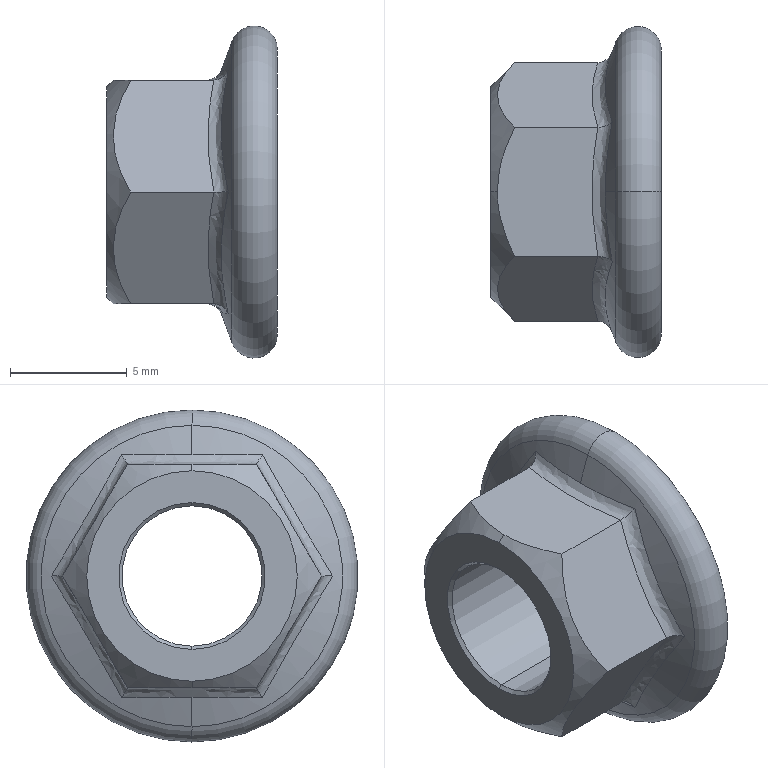Part | SolidWorks | features Cut 2, Boss 1, Chamfer 1, Fillet 1, Revolution 1 | 1 solid | 26 faces | box 7.3 x 14.2 x 14.2 mm | volume 518.031 mm3 | cone 8 | plane 8 | spline 6 | cylinder 2 | torus 2 | commonest cylinder face diameters 6 x2
STEP:
#1=CARTESIAN_POINT('',(-7.3,0.,-4.5));
#2=VERTEX_POINT('',#1);
#3=CARTESIAN_POINT('',(-7.3,0.,4.5));
#4=VERTEX_POINT('',#3);
#5=CARTESIAN_POINT('',(-7.3,0.,0.));
#6=DIRECTION('',(-1.,0.,0.));
#7=DIRECTION('',(0.,0.,1.));
#8=AXIS2_PLACEMENT_3D('',#5,#6,#7);
#9=CIRCLE('',#8,4.5);
#10=EDGE_CURVE('',#2,#4,#9,.T.);
#11=ORIENTED_EDGE('',*,*,#10,.F.);
#12=CARTESIAN_POINT('',(-7.015,0.,-4.785));
#13=VERTEX_POINT('',#12);
#14=CARTESIAN_POINT('',(-7.3,0.,-4.5));
#15=DIRECTION('',(0.7071,0.,-0.7071));
#16=VECTOR('',#15,1000.);
#17=LINE('',#14,#16);
#18=EDGE_CURVE('',#2,#13,#17,.T.);
#19=ORIENTED_EDGE('',*,*,#18,.T.);
#20=CARTESIAN_POINT('',(-6.275,-2.762,-4.785));
#21=VERTEX_POINT('',#20);
#22=CARTESIAN_POINT('',(-7.015,0.,-4.785));
#23=CARTESIAN_POINT('',(-7.015,-0.2426,-4.785));
#24=CARTESIAN_POINT('',(-6.996,-0.4848,-4.785));
#25=CARTESIAN_POINT('',(-6.926,-0.9587,-4.785));
#26=CARTESIAN_POINT('',(-6.874,-1.192,-4.785));
#27=CARTESIAN_POINT('',(-6.677,-1.883,-4.785));
#28=CARTESIAN_POINT('',(-6.489,-2.334,-4.785));
#29=CARTESIAN_POINT('',(-6.275,-2.762,-4.785));
#30=B_SPLINE_CURVE_WITH_KNOTS('',3,(#22,#23,#24,#25,#26,#27,#28,#29),.UNSPECIFIED.,.F.,.F.,(4,2,2,4),(0.005791,0.006506,0.007221,0.008651),.UNSPECIFIED.);
#31=EDGE_CURVE('',#13,#21,#30,.T.);
#32=ORIENTED_EDGE('',*,*,#31,.T.);
#33=CARTESIAN_POINT('',(-6.275,-5.525,0.));
#34=VERTEX_POINT('',#33);
#35=CARTESIAN_POINT('',(-6.275,-2.762,-4.785));
#36=CARTESIAN_POINT('',(-6.491,-2.978,-4.411));
#37=CARTESIAN_POINT('',(-6.674,-3.199,-4.029));
#38=CARTESIAN_POINT('',(-6.871,-3.542,-3.435));
#39=CARTESIAN_POINT('',(-6.923,-3.658,-3.233));
#40=CARTESIAN_POINT('',(-6.995,-3.896,-2.822));
#41=CARTESIAN_POINT('',(-7.015,-4.018,-2.61));
#42=CARTESIAN_POINT('',(-7.016,-4.38,-1.984));
#43=CARTESIAN_POINT('',(-6.943,-4.617,-1.573));
#44=CARTESIAN_POINT('',(-6.678,-5.084,-0.7632));
#45=CARTESIAN_POINT('',(-6.492,-5.308,-0.376));
#46=CARTESIAN_POINT('',(-6.275,-5.525,0.));
#47=B_SPLINE_CURVE_WITH_KNOTS('',3,(#35,#36,#37,#38,#39,#40,#41,#42,#43,#44,#45,#46),.UNSPECIFIED.,.F.,.F.,(4,2,2,2,2,4),(0.000000254,0.001427,0.00214,0.002854,0.004281,0.005707),.UNSPECIFIED.);
#48=EDGE_CURVE('',#21,#34,#47,.T.);
#49=ORIENTED_EDGE('',*,*,#48,.T.);
#50=CARTESIAN_POINT('',(-6.275,-2.763,4.785));
#51=VERTEX_POINT('',#50);
#52=CARTESIAN_POINT('',(-6.275,-5.525,0.));
#53=CARTESIAN_POINT('',(-6.491,-5.309,0.3738));
#54=CARTESIAN_POINT('',(-6.674,-5.088,0.7561));
#55=CARTESIAN_POINT('',(-6.871,-4.746,1.35));
#56=CARTESIAN_POINT('',(-6.923,-4.629,1.551));
#57=CARTESIAN_POINT('',(-6.995,-4.392,1.963));
#58=CARTESIAN_POINT('',(-7.015,-4.269,2.175));
#59=CARTESIAN_POINT('',(-7.016,-3.908,2.801));
#60=CARTESIAN_POINT('',(-6.943,-3.671,3.212));
#61=CARTESIAN_POINT('',(-6.678,-3.203,4.022));
#62=CARTESIAN_POINT('',(-6.492,-2.98,4.409));
#63=CARTESIAN_POINT('',(-6.275,-2.763,4.785));
#64=B_SPLINE_CURVE_WITH_KNOTS('',3,(#52,#53,#54,#55,#56,#57,#58,#59,#60,#61,#62,#63),.UNSPECIFIED.,.F.,.F.,(4,2,2,2,2,4),(0.000000254,0.001427,0.00214,0.002854,0.004281,0.005707),.UNSPECIFIED.);
#65=EDGE_CURVE('',#34,#51,#64,.T.);
#66=ORIENTED_EDGE('',*,*,#65,.T.);
#67=CARTESIAN_POINT('',(-7.015,0.,4.785));
#68=VERTEX_POINT('',#67);
#69=CARTESIAN_POINT('',(-6.275,-2.763,4.785));
#70=CARTESIAN_POINT('',(-6.489,-2.334,4.785));
#71=CARTESIAN_POINT('',(-6.677,-1.883,4.785));
#72=CARTESIAN_POINT('',(-6.874,-1.192,4.785));
#73=CARTESIAN_POINT('',(-6.926,-0.9587,4.785));
#74=CARTESIAN_POINT('',(-6.996,-0.4848,4.785));
#75=CARTESIAN_POINT('',(-7.015,-0.2426,4.785));
#76=CARTESIAN_POINT('',(-7.015,0.,4.785));
#77=B_SPLINE_CURVE_WITH_KNOTS('',3,(#69,#70,#71,#72,#73,#74,#75,#76),.UNSPECIFIED.,.F.,.F.,(4,2,2,4),(0.00366,0.005092,0.005807,0.006523),.UNSPECIFIED.);
#78=EDGE_CURVE('',#51,#68,#77,.T.);
#79=ORIENTED_EDGE('',*,*,#78,.T.);
#80=CARTESIAN_POINT('',(-7.3,0.,4.5));
#81=DIRECTION('',(0.7071,0.,0.7071));
#82=VECTOR('',#81,1000.);
#83=LINE('',#80,#82);
#84=EDGE_CURVE('',#4,#68,#83,.T.);
#85=ORIENTED_EDGE('',*,*,#84,.F.);
#86=EDGE_LOOP('',(#11,#19,#32,#49,#66,#79,#85));
#87=FACE_OUTER_BOUND('',#86,.T.);
#88=CARTESIAN_POINT('',(-7.3,0.,0.));
#89=DIRECTION('',(1.,0.,0.));
#90=DIRECTION('',(0.,0.,1.));
#91=AXIS2_PLACEMENT_3D('',#88,#89,#90);
#92=CONICAL_SURFACE('',#91,4.5,0.7854);
#93=ADVANCED_FACE('',(#87),#92,.T.);
#94=CARTESIAN_POINT('',(-0.1429,0.,3.));
#95=VERTEX_POINT('',#94);
#96=CARTESIAN_POINT('',(-0.1429,0.,-3.));
#97=VERTEX_POINT('',#96);
#98=CARTESIAN_POINT('',(-0.1429,0.,0.));
#99=DIRECTION('',(1.,0.,0.));
#100=DIRECTION('',(0.,0.,1.));
#101=AXIS2_PLACEMENT_3D('',#98,#99,#100);
#102=CIRCLE('',#101,3.);
#103=EDGE_CURVE('',#95,#97,#102,.T.);
#104=ORIENTED_EDGE('',*,*,#103,.F.);
#105=CARTESIAN_POINT('',(0.,0.,3.143));
#106=VERTEX_POINT('',#105);
#107=CARTESIAN_POINT('',(0.,0.,3.143));
#108=DIRECTION('',(0.7071,0.,0.7071));
#109=VECTOR('',#108,1000.);
#110=LINE('',#107,#109);
#111=EDGE_CURVE('',#95,#106,#110,.T.);
#112=ORIENTED_EDGE('',*,*,#111,.T.);
#113=CARTESIAN_POINT('',(0.,0.,-3.143));
#114=VERTEX_POINT('',#113);
#115=CARTESIAN_POINT('',(0.,0.,0.));
#116=DIRECTION('',(-1.,0.,0.));
#117=DIRECTION('',(0.,0.,1.));
#118=AXIS2_PLACEMENT_3D('',#115,#116,#117);
#119=CIRCLE('',#118,3.143);
#120=EDGE_CURVE('',#114,#106,#119,.T.);
#121=ORIENTED_EDGE('',*,*,#120,.F.);
#122=CARTESIAN_POINT('',(0.,0.,-3.143));
#123=DIRECTION('',(0.7071,0.,-0.7071));
#124=VECTOR('',#123,1000.);
#125=LINE('',#122,#124);
#126=EDGE_CURVE('',#97,#114,#125,.T.);
#127=ORIENTED_EDGE('',*,*,#126,.F.);
#128=EDGE_LOOP('',(#104,#112,#121,#127));
#129=FACE_OUTER_BOUND('',#128,.T.);
#130=CARTESIAN_POINT('',(0.,0.,0.));
#131=DIRECTION('',(1.,0.,0.));
#132=DIRECTION('',(0.,0.,-1.));
#133=AXIS2_PLACEMENT_3D('',#130,#131,#132);
#134=CONICAL_SURFACE('',#133,3.143,0.7854);
#135=ADVANCED_FACE('',(#129),#134,.F.);
#136=CARTESIAN_POINT('',(-7.157,0.,-3.));
#137=VERTEX_POINT('',#136);
#138=CARTESIAN_POINT('',(-7.157,0.,3.));
#139=VERTEX_POINT('',#138);
#140=CARTESIAN_POINT('',(-7.157,0.,0.));
#141=DIRECTION('',(-1.,0.,0.));
#142=DIRECTION('',(0.,0.,-1.));
#143=AXIS2_PLACEMENT_3D('',#140,#141,#142);
#144=CIRCLE('',#143,3.);
#145=EDGE_CURVE('',#137,#139,#144,.T.);
#146=ORIENTED_EDGE('',*,*,#145,.F.);
#147=CARTESIAN_POINT('',(-7.3,0.,-3.143));
#148=VERTEX_POINT('',#147);
#149=CARTESIAN_POINT('',(-7.157,0.,-3.));
#150=DIRECTION('',(-0.7071,0.,-0.7071));
#151=VECTOR('',#150,1000.);
#152=LINE('',#149,#151);
#153=EDGE_CURVE('',#137,#148,#152,.T.);
#154=ORIENTED_EDGE('',*,*,#153,.T.);
#155=CARTESIAN_POINT('',(-7.3,0.,3.143));
#156=VERTEX_POINT('',#155);
#157=CARTESIAN_POINT('',(-7.3,0.,0.));
#158=DIRECTION('',(1.,0.,0.));
#159=DIRECTION('',(0.,0.,-1.));
#160=AXIS2_PLACEMENT_3D('',#157,#158,#159);
#161=CIRCLE('',#160,3.143);
#162=EDGE_CURVE('',#156,#148,#161,.T.);
#163=ORIENTED_EDGE('',*,*,#162,.F.);
#164=CARTESIAN_POINT('',(-7.157,0.,3.));
#165=DIRECTION('',(-0.7071,0.,0.7071));
#166=VECTOR('',#165,1000.);
#167=LINE('',#164,#166);
#168=EDGE_CURVE('',#139,#156,#167,.T.);
#169=ORIENTED_EDGE('',*,*,#168,.F.);
#170=EDGE_LOOP('',(#146,#154,#163,#169));
#171=FACE_OUTER_BOUND('',#170,.T.);
#172=CARTESIAN_POINT('',(-7.157,0.,0.));
#173=DIRECTION('',(-1.,0.,0.));
#174=DIRECTION('',(0.,0.,1.));
#175=AXIS2_PLACEMENT_3D('',#172,#173,#174);
#176=CONICAL_SURFACE('',#175,3.,0.7854);
#177=ADVANCED_FACE('',(#171),#176,.F.);
#178=ORIENTED_EDGE('',*,*,#103,.T.);
#179=CARTESIAN_POINT('',(0.,0.,-3.));
#180=DIRECTION('',(-1.,0.,0.));
#181=VECTOR('',#180,1000.);
#182=LINE('',#179,#181);
#183=EDGE_CURVE('',#97,#137,#182,.T.);
#184=ORIENTED_EDGE('',*,*,#183,.T.);
#185=ORIENTED_EDGE('',*,*,#145,.T.);
#186=CARTESIAN_POINT('',(0.,0.,3.));
#187=DIRECTION('',(-1.,0.,0.));
#188=VECTOR('',#187,1000.);
#189=LINE('',#186,#188);
#190=EDGE_CURVE('',#95,#139,#189,.T.);
#191=ORIENTED_EDGE('',*,*,#190,.F.);
#192=EDGE_LOOP('',(#178,#184,#185,#191));
#193=FACE_OUTER_BOUND('',#192,.T.);
#194=CARTESIAN_POINT('',(0.,0.,0.));
#195=DIRECTION('',(-1.,0.,0.));
#196=DIRECTION('',(0.,0.,1.));
#197=AXIS2_PLACEMENT_3D('',#194,#195,#196);
#198=CYLINDRICAL_SURFACE('',#197,3.);
#199=ADVANCED_FACE('',(#193),#198,.F.);
#200=CARTESIAN_POINT('',(0.,0.,6.1));
#201=VERTEX_POINT('',#200);
#202=CARTESIAN_POINT('',(0.,0.,-6.1));
#203=VERTEX_POINT('',#202);
#204=CARTESIAN_POINT('',(0.,0.,0.));
#205=DIRECTION('',(-1.,0.,0.));
#206=DIRECTION('',(0.,0.,1.));
#207=AXIS2_PLACEMENT_3D('',#204,#205,#206);
#208=CIRCLE('',#207,6.1);
#209=EDGE_CURVE('',#201,#203,#208,.T.);
#210=ORIENTED_EDGE('',*,*,#209,.T.);
#211=CARTESIAN_POINT('',(-1.94,0.,-6.442));
#212=VERTEX_POINT('',#211);
#213=CARTESIAN_POINT('',(-1.,0.,-6.1));
#214=DIRECTION('',(0.,1.,0.));
#215=DIRECTION('',(0.,0.,1.));
#216=AXIS2_PLACEMENT_3D('',#213,#214,#215);
#217=CIRCLE('',#216,1.);
#218=EDGE_CURVE('',#203,#212,#217,.T.);
#219=ORIENTED_EDGE('',*,*,#218,.T.);
#220=CARTESIAN_POINT('',(-1.94,0.,6.442));
#221=VERTEX_POINT('',#220);
#222=CARTESIAN_POINT('',(-1.94,0.,0.));
#223=DIRECTION('',(-1.,0.,0.));
#224=DIRECTION('',(0.,0.,1.));
#225=AXIS2_PLACEMENT_3D('',#222,#223,#224);
#226=CIRCLE('',#225,6.442);
#227=EDGE_CURVE('',#221,#212,#226,.T.);
#228=ORIENTED_EDGE('',*,*,#227,.F.);
#229=CARTESIAN_POINT('',(-1.,0.,6.1));
#230=DIRECTION('',(0.,-1.,0.));
#231=DIRECTION('',(0.,0.,-1.));
#232=AXIS2_PLACEMENT_3D('',#229,#230,#231);
#233=CIRCLE('',#232,1.);
#234=EDGE_CURVE('',#201,#221,#233,.T.);
#235=ORIENTED_EDGE('',*,*,#234,.F.);
#236=EDGE_LOOP('',(#210,#219,#228,#235));
#237=FACE_OUTER_BOUND('',#236,.T.);
#238=CARTESIAN_POINT('',(-1.,0.,0.));
#239=DIRECTION('',(-1.,0.,0.));
#240=DIRECTION('',(0.,0.,1.));
#241=AXIS2_PLACEMENT_3D('',#238,#239,#240);
#242=TOROIDAL_SURFACE('',#241,6.1,1.);
#243=ADVANCED_FACE('',(#237),#242,.T.);
#244=CARTESIAN_POINT('',(-2.096,3.006,5.207));
#245=VERTEX_POINT('',#244);
#246=CARTESIAN_POINT('',(-2.399,0.,5.18));
#247=VERTEX_POINT('',#246);
#248=CARTESIAN_POINT('',(-2.096,3.006,5.207));
#249=CARTESIAN_POINT('',(-2.281,2.013,5.193));
#250=CARTESIAN_POINT('',(-2.399,1.012,5.18));
#251=CARTESIAN_POINT('',(-2.399,0.,5.18));
#252=B_SPLINE_CURVE_WITH_KNOTS('',3,(#248,#249,#250,#251),.UNSPECIFIED.,.F.,.F.,(4,4),(0.,0.003022),.UNSPECIFIED.);
#253=EDGE_CURVE('',#245,#247,#252,.T.);
#254=ORIENTED_EDGE('',*,*,#253,.T.);
#255=CARTESIAN_POINT('',(-1.94,0.,6.442));
#256=DIRECTION('',(0.342,0.,0.9397));
#257=VECTOR('',#256,1000.);
#258=LINE('',#255,#257);
#259=EDGE_CURVE('',#247,#221,#258,.T.);
#260=ORIENTED_EDGE('',*,*,#259,.T.);
#261=ORIENTED_EDGE('',*,*,#227,.T.);
#262=CARTESIAN_POINT('',(-2.399,0.,-5.18));
#263=VERTEX_POINT('',#262);
#264=CARTESIAN_POINT('',(-1.94,0.,-6.442));
#265=DIRECTION('',(0.342,0.,-0.9397));
#266=VECTOR('',#265,1000.);
#267=LINE('',#264,#266);
#268=EDGE_CURVE('',#263,#212,#267,.T.);
#269=ORIENTED_EDGE('',*,*,#268,.F.);
#270=CARTESIAN_POINT('',(-2.096,3.006,-5.207));
#271=VERTEX_POINT('',#270);
#272=CARTESIAN_POINT('',(-2.399,0.,-5.18));
#273=CARTESIAN_POINT('',(-2.399,0.5051,-5.18));
#274=CARTESIAN_POINT('',(-2.371,1.008,-5.183));
#275=CARTESIAN_POINT('',(-2.265,2.01,-5.193));
#276=CARTESIAN_POINT('',(-2.189,2.51,-5.2));
#277=CARTESIAN_POINT('',(-2.096,3.006,-5.207));
#278=B_SPLINE_CURVE_WITH_KNOTS('',3,(#272,#273,#274,#275,#276,#277),.UNSPECIFIED.,.F.,.F.,(4,2,4),(0.003022,0.004529,0.006037),.UNSPECIFIED.);
#279=EDGE_CURVE('',#263,#271,#278,.T.);
#280=ORIENTED_EDGE('',*,*,#279,.T.);
#281=CARTESIAN_POINT('',(-2.096,6.013,0.));
#282=VERTEX_POINT('',#281);
#283=CARTESIAN_POINT('',(-2.096,3.006,-5.207));
#284=CARTESIAN_POINT('',(-2.281,3.49,-4.34));
#285=CARTESIAN_POINT('',(-2.399,3.978,-3.468));
#286=CARTESIAN_POINT('',(-2.399,4.737,-2.155));
#287=CARTESIAN_POINT('',(-2.371,4.991,-1.72));
#288=CARTESIAN_POINT('',(-2.265,5.502,-0.8562));
#289=CARTESIAN_POINT('',(-2.189,5.758,-0.4266));
#290=CARTESIAN_POINT('',(-2.096,6.013,0.));
#291=B_SPLINE_CURVE_WITH_KNOTS('',3,(#283,#284,#285,#286,#287,#288,#289,#290),.UNSPECIFIED.,.F.,.F.,(4,2,2,4),(0.,0.003019,0.004528,0.006037),.UNSPECIFIED.);
#292=EDGE_CURVE('',#271,#282,#291,.T.);
#293=ORIENTED_EDGE('',*,*,#292,.T.);
#294=CARTESIAN_POINT('',(-2.096,6.013,0.));
#295=CARTESIAN_POINT('',(-2.281,5.504,0.8523));
#296=CARTESIAN_POINT('',(-2.399,4.993,1.711));
#297=CARTESIAN_POINT('',(-2.399,4.234,3.025));
#298=CARTESIAN_POINT('',(-2.371,3.985,3.463));
#299=CARTESIAN_POINT('',(-2.265,3.492,4.337));
#300=CARTESIAN_POINT('',(-2.189,3.248,4.773));
#301=CARTESIAN_POINT('',(-2.096,3.006,5.207));
#302=B_SPLINE_CURVE_WITH_KNOTS('',3,(#294,#295,#296,#297,#298,#299,#300,#301),.UNSPECIFIED.,.F.,.F.,(4,2,2,4),(0.,0.003019,0.004528,0.006037),.UNSPECIFIED.);
#303=EDGE_CURVE('',#282,#245,#302,.T.);
#304=ORIENTED_EDGE('',*,*,#303,.T.);
#305=EDGE_LOOP('',(#254,#260,#261,#269,#280,#293,#304));
#306=FACE_OUTER_BOUND('',#305,.T.);
#307=CARTESIAN_POINT('',(-1.94,0.,0.));
#308=DIRECTION('',(1.,0.,0.));
#309=DIRECTION('',(0.,0.,-1.));
#310=AXIS2_PLACEMENT_3D('',#307,#308,#309);
#311=CONICAL_SURFACE('',#310,6.442,1.222);
#312=ADVANCED_FACE('',(#306),#311,.T.);
#313=CARTESIAN_POINT('',(-6.275,2.763,4.785));
#314=VERTEX_POINT('',#313);
#315=CARTESIAN_POINT('',(-2.72,2.763,4.785));
#316=VERTEX_POINT('',#315);
#317=CARTESIAN_POINT('',(-7.3,2.763,4.785));
#318=DIRECTION('',(1.,0.,0.));
#319=VECTOR('',#318,1000.);
#320=LINE('',#317,#319);
#321=EDGE_CURVE('',#314,#316,#320,.T.);
#322=ORIENTED_EDGE('',*,*,#321,.T.);
#323=CARTESIAN_POINT('',(-2.72,5.525,0.));
#324=VERTEX_POINT('',#323);
#325=CARTESIAN_POINT('',(-2.72,2.763,4.785));
#326=CARTESIAN_POINT('',(-2.872,3.22,3.993));
#327=CARTESIAN_POINT('',(-2.963,3.68,3.196));
#328=CARTESIAN_POINT('',(-2.963,4.608,1.589));
#329=CARTESIAN_POINT('',(-2.872,5.068,0.7921));
#330=CARTESIAN_POINT('',(-2.72,5.525,0.));
#331=B_SPLINE_CURVE_WITH_KNOTS('',3,(#325,#326,#327,#328,#329,#330),.UNSPECIFIED.,.F.,.F.,(4,2,4),(0.,0.002773,0.005546),.UNSPECIFIED.);
#332=EDGE_CURVE('',#316,#324,#331,.T.);
#333=ORIENTED_EDGE('',*,*,#332,.T.);
#334=CARTESIAN_POINT('',(-6.275,5.525,0.));
#335=VERTEX_POINT('',#334);
#336=CARTESIAN_POINT('',(-7.3,5.525,0.));
#337=DIRECTION('',(1.,0.,0.));
#338=VECTOR('',#337,1000.);
#339=LINE('',#336,#338);
#340=EDGE_CURVE('',#335,#324,#339,.T.);
#341=ORIENTED_EDGE('',*,*,#340,.F.);
#342=CARTESIAN_POINT('',(-6.275,2.763,4.785));
#343=CARTESIAN_POINT('',(-6.491,2.978,4.411));
#344=CARTESIAN_POINT('',(-6.674,3.199,4.029));
#345=CARTESIAN_POINT('',(-6.871,3.542,3.435));
#346=CARTESIAN_POINT('',(-6.923,3.658,3.233));
#347=CARTESIAN_POINT('',(-6.995,3.896,2.822));
#348=CARTESIAN_POINT('',(-7.015,4.018,2.61));
#349=CARTESIAN_POINT('',(-7.016,4.38,1.984));
#350=CARTESIAN_POINT('',(-6.943,4.617,1.573));
#351=CARTESIAN_POINT('',(-6.678,5.084,0.7632));
#352=CARTESIAN_POINT('',(-6.492,5.308,0.376));
#353=CARTESIAN_POINT('',(-6.275,5.525,0.));
#354=B_SPLINE_CURVE_WITH_KNOTS('',3,(#342,#343,#344,#345,#346,#347,#348,#349,#350,#351,#352,#353),.UNSPECIFIED.,.F.,.F.,(4,2,2,2,2,4),(0.000000254,0.001427,0.00214,0.002854,0.004281,0.005707),.UNSPECIFIED.);
#355=EDGE_CURVE('',#314,#335,#354,.T.);
#356=ORIENTED_EDGE('',*,*,#355,.F.);
#357=EDGE_LOOP('',(#322,#333,#341,#356));
#358=FACE_OUTER_BOUND('',#357,.T.);
#359=CARTESIAN_POINT('',(-7.3,2.763,4.785));
#360=DIRECTION('',(0.,-0.866,-0.5));
#361=DIRECTION('',(0.,0.5,-0.866));
#362=AXIS2_PLACEMENT_3D('',#359,#360,#361);
#363=PLANE('',#362);
#364=ADVANCED_FACE('',(#358),#363,.F.);
#365=ORIENTED_EDGE('',*,*,#340,.T.);
#366=CARTESIAN_POINT('',(-2.72,2.763,-4.785));
#367=VERTEX_POINT('',#366);
#368=CARTESIAN_POINT('',(-2.72,5.525,0.));
#369=CARTESIAN_POINT('',(-2.872,5.068,-0.7921));
#370=CARTESIAN_POINT('',(-2.963,4.608,-1.589));
#371=CARTESIAN_POINT('',(-2.963,3.68,-3.196));
#372=CARTESIAN_POINT('',(-2.872,3.22,-3.993));
#373=CARTESIAN_POINT('',(-2.72,2.763,-4.785));
#374=B_SPLINE_CURVE_WITH_KNOTS('',3,(#368,#369,#370,#371,#372,#373),.UNSPECIFIED.,.F.,.F.,(4,2,4),(0.,0.002773,0.005546),.UNSPECIFIED.);
#375=EDGE_CURVE('',#324,#367,#374,.T.);
#376=ORIENTED_EDGE('',*,*,#375,.T.);
#377=CARTESIAN_POINT('',(-6.275,2.763,-4.785));
#378=VERTEX_POINT('',#377);
#379=CARTESIAN_POINT('',(-7.3,2.763,-4.785));
#380=DIRECTION('',(1.,0.,0.));
#381=VECTOR('',#380,1000.);
#382=LINE('',#379,#381);
#383=EDGE_CURVE('',#378,#367,#382,.T.);
#384=ORIENTED_EDGE('',*,*,#383,.F.);
#385=CARTESIAN_POINT('',(-6.275,5.525,0.));
#386=CARTESIAN_POINT('',(-6.491,5.309,-0.3738));
#387=CARTESIAN_POINT('',(-6.674,5.088,-0.7561));
#388=CARTESIAN_POINT('',(-6.871,4.746,-1.35));
#389=CARTESIAN_POINT('',(-6.923,4.629,-1.551));
#390=CARTESIAN_POINT('',(-6.995,4.392,-1.963));
#391=CARTESIAN_POINT('',(-7.015,4.269,-2.175));
#392=CARTESIAN_POINT('',(-7.016,3.908,-2.801));
#393=CARTESIAN_POINT('',(-6.943,3.671,-3.212));
#394=CARTESIAN_POINT('',(-6.678,3.203,-4.022));
#395=CARTESIAN_POINT('',(-6.492,2.98,-4.409));
#396=CARTESIAN_POINT('',(-6.275,2.763,-4.785));
#397=B_SPLINE_CURVE_WITH_KNOTS('',3,(#385,#386,#387,#388,#389,#390,#391,#392,#393,#394,#395,#396),.UNSPECIFIED.,.F.,.F.,(4,2,2,2,2,4),(0.000000254,0.001427,0.00214,0.002854,0.004281,0.005707),.UNSPECIFIED.);
#398=EDGE_CURVE('',#335,#378,#397,.T.);
#399=ORIENTED_EDGE('',*,*,#398,.F.);
#400=EDGE_LOOP('',(#365,#376,#384,#399));
#401=FACE_OUTER_BOUND('',#400,.T.);
#402=CARTESIAN_POINT('',(-7.3,5.525,0.));
#403=DIRECTION('',(0.,-0.866,0.5));
#404=DIRECTION('',(0.,-0.5,-0.866));
#405=AXIS2_PLACEMENT_3D('',#402,#403,#404);
#406=PLANE('',#405);
#407=ADVANCED_FACE('',(#401),#406,.F.);
#408=ORIENTED_EDGE('',*,*,#383,.T.);
#409=CARTESIAN_POINT('',(-2.72,-2.762,-4.785));
#410=VERTEX_POINT('',#409);
#411=CARTESIAN_POINT('',(-2.72,2.763,-4.785));
#412=CARTESIAN_POINT('',(-2.872,1.848,-4.785));
#413=CARTESIAN_POINT('',(-2.963,0.9279,-4.785));
#414=CARTESIAN_POINT('',(-2.963,-0.928,-4.785));
#415=CARTESIAN_POINT('',(-2.872,-1.848,-4.785));
#416=CARTESIAN_POINT('',(-2.72,-2.762,-4.785));
#417=B_SPLINE_CURVE_WITH_KNOTS('',3,(#411,#412,#413,#414,#415,#416),.UNSPECIFIED.,.F.,.F.,(4,2,4),(0.,0.002773,0.005546),.UNSPECIFIED.);
#418=EDGE_CURVE('',#367,#410,#417,.T.);
#419=ORIENTED_EDGE('',*,*,#418,.T.);
#420=CARTESIAN_POINT('',(-7.3,-2.762,-4.785));
#421=DIRECTION('',(1.,0.,0.));
#422=VECTOR('',#421,1000.);
#423=LINE('',#420,#422);
#424=EDGE_CURVE('',#21,#410,#423,.T.);
#425=ORIENTED_EDGE('',*,*,#424,.F.);
#426=ORIENTED_EDGE('',*,*,#31,.F.);
#427=CARTESIAN_POINT('',(-6.275,2.763,-4.785));
#428=CARTESIAN_POINT('',(-6.382,2.549,-4.785));
#429=CARTESIAN_POINT('',(-6.482,2.331,-4.785));
#430=CARTESIAN_POINT('',(-6.662,1.884,-4.785));
#431=CARTESIAN_POINT('',(-6.742,1.653,-4.785));
#432=CARTESIAN_POINT('',(-6.94,0.9586,-4.785));
#433=CARTESIAN_POINT('',(-7.015,0.4856,-4.785));
#434=CARTESIAN_POINT('',(-7.015,0.,-4.785));
#435=B_SPLINE_CURVE_WITH_KNOTS('',3,(#427,#428,#429,#430,#431,#432,#433,#434),.UNSPECIFIED.,.F.,.F.,(4,2,2,4),(0.002927,0.003643,0.004359,0.005791),.UNSPECIFIED.);
#436=EDGE_CURVE('',#378,#13,#435,.T.);
#437=ORIENTED_EDGE('',*,*,#436,.F.);
#438=EDGE_LOOP('',(#408,#419,#425,#426,#437));
#439=FACE_OUTER_BOUND('',#438,.T.);
#440=CARTESIAN_POINT('',(-7.3,2.763,-4.785));
#441=DIRECTION('',(0.,0.,1.));
#442=DIRECTION('',(0.,-1.,0.));
#443=AXIS2_PLACEMENT_3D('',#440,#441,#442);
#444=PLANE('',#443);
#445=ADVANCED_FACE('',(#439),#444,.F.);
#446=ORIENTED_EDGE('',*,*,#424,.T.);
#447=CARTESIAN_POINT('',(-2.72,-5.525,0.));
#448=VERTEX_POINT('',#447);
#449=CARTESIAN_POINT('',(-2.72,-2.762,-4.785));
#450=CARTESIAN_POINT('',(-2.872,-3.22,-3.993));
#451=CARTESIAN_POINT('',(-2.963,-3.68,-3.196));
#452=CARTESIAN_POINT('',(-2.963,-4.608,-1.589));
#453=CARTESIAN_POINT('',(-2.872,-5.068,-0.7921));
#454=CARTESIAN_POINT('',(-2.72,-5.525,0.));
#455=B_SPLINE_CURVE_WITH_KNOTS('',3,(#449,#450,#451,#452,#453,#454),.UNSPECIFIED.,.F.,.F.,(4,2,4),(0.,0.002773,0.005546),.UNSPECIFIED.);
#456=EDGE_CURVE('',#410,#448,#455,.T.);
#457=ORIENTED_EDGE('',*,*,#456,.T.);
#458=CARTESIAN_POINT('',(-7.3,-5.525,0.));
#459=DIRECTION('',(1.,0.,0.));
#460=VECTOR('',#459,1000.);
#461=LINE('',#458,#460);
#462=EDGE_CURVE('',#34,#448,#461,.T.);
#463=ORIENTED_EDGE('',*,*,#462,.F.);
#464=ORIENTED_EDGE('',*,*,#48,.F.);
#465=EDGE_LOOP('',(#446,#457,#463,#464));
#466=FACE_OUTER_BOUND('',#465,.T.);
#467=CARTESIAN_POINT('',(-7.3,-2.762,-4.785));
#468=DIRECTION('',(0.,0.866,0.5));
#469=DIRECTION('',(0.,-0.5,0.866));
#470=AXIS2_PLACEMENT_3D('',#467,#468,#469);
#471=PLANE('',#470);
#472=ADVANCED_FACE('',(#466),#471,.F.);
#473=ORIENTED_EDGE('',*,*,#462,.T.);
#474=CARTESIAN_POINT('',(-2.72,-2.763,4.785));
#475=VERTEX_POINT('',#474);
#476=CARTESIAN_POINT('',(-2.72,-5.525,0.));
#477=CARTESIAN_POINT('',(-2.872,-5.068,0.7921));
#478=CARTESIAN_POINT('',(-2.963,-4.608,1.589));
#479=CARTESIAN_POINT('',(-2.963,-3.68,3.196));
#480=CARTESIAN_POINT('',(-2.872,-3.22,3.993));
#481=CARTESIAN_POINT('',(-2.72,-2.763,4.785));
#482=B_SPLINE_CURVE_WITH_KNOTS('',3,(#476,#477,#478,#479,#480,#481),.UNSPECIFIED.,.F.,.F.,(4,2,4),(0.,0.002773,0.005546),.UNSPECIFIED.);
#483=EDGE_CURVE('',#448,#475,#482,.T.);
#484=ORIENTED_EDGE('',*,*,#483,.T.);
#485=CARTESIAN_POINT('',(-7.3,-2.763,4.785));
#486=DIRECTION('',(1.,0.,0.));
#487=VECTOR('',#486,1000.);
#488=LINE('',#485,#487);
#489=EDGE_CURVE('',#51,#475,#488,.T.);
#490=ORIENTED_EDGE('',*,*,#489,.F.);
#491=ORIENTED_EDGE('',*,*,#65,.F.);
#492=EDGE_LOOP('',(#473,#484,#490,#491));
#493=FACE_OUTER_BOUND('',#492,.T.);
#494=CARTESIAN_POINT('',(-7.3,-5.525,0.));
#495=DIRECTION('',(0.,0.866,-0.5));
#496=DIRECTION('',(0.,0.5,0.866));
#497=AXIS2_PLACEMENT_3D('',#494,#495,#496);
#498=PLANE('',#497);
#499=ADVANCED_FACE('',(#493),#498,.F.);
#500=ORIENTED_EDGE('',*,*,#489,.T.);
#501=CARTESIAN_POINT('',(-2.72,-2.763,4.785));
#502=CARTESIAN_POINT('',(-2.872,-1.848,4.785));
#503=CARTESIAN_POINT('',(-2.963,-0.928,4.785));
#504=CARTESIAN_POINT('',(-2.963,0.9279,4.785));
#505=CARTESIAN_POINT('',(-2.872,1.848,4.785));
#506=CARTESIAN_POINT('',(-2.72,2.763,4.785));
#507=B_SPLINE_CURVE_WITH_KNOTS('',3,(#501,#502,#503,#504,#505,#506),.UNSPECIFIED.,.F.,.F.,(4,2,4),(0.,0.002773,0.005546),.UNSPECIFIED.);
#508=EDGE_CURVE('',#475,#316,#507,.T.);
#509=ORIENTED_EDGE('',*,*,#508,.T.);
#510=ORIENTED_EDGE('',*,*,#321,.F.);
#511=CARTESIAN_POINT('',(-7.015,0.,4.785));
#512=CARTESIAN_POINT('',(-7.015,0.4856,4.785));
#513=CARTESIAN_POINT('',(-6.94,0.9586,4.785));
#514=CARTESIAN_POINT('',(-6.742,1.653,4.785));
#515=CARTESIAN_POINT('',(-6.662,1.884,4.785));
#516=CARTESIAN_POINT('',(-6.482,2.331,4.785));
#517=CARTESIAN_POINT('',(-6.382,2.549,4.785));
#518=CARTESIAN_POINT('',(-6.275,2.763,4.785));
#519=B_SPLINE_CURVE_WITH_KNOTS('',3,(#511,#512,#513,#514,#515,#516,#517,#518),.UNSPECIFIED.,.F.,.F.,(4,2,2,4),(0.006523,0.007956,0.008672,0.009389),.UNSPECIFIED.);
#520=EDGE_CURVE('',#68,#314,#519,.T.);
#521=ORIENTED_EDGE('',*,*,#520,.F.);
#522=ORIENTED_EDGE('',*,*,#78,.F.);
#523=EDGE_LOOP('',(#500,#509,#510,#521,#522));
#524=FACE_OUTER_BOUND('',#523,.T.);
#525=CARTESIAN_POINT('',(-7.3,-2.763,4.785));
#526=DIRECTION('',(0.,0.,-1.));
#527=DIRECTION('',(0.,1.,0.));
#528=AXIS2_PLACEMENT_3D('',#525,#526,#527);
#529=PLANE('',#528);
#530=ADVANCED_FACE('',(#524),#529,.F.);
#531=ORIENTED_EDGE('',*,*,#162,.T.);
#532=CARTESIAN_POINT('',(-7.3,0.,0.));
#533=DIRECTION('',(1.,0.,0.));
#534=DIRECTION('',(0.,0.,-1.));
#535=AXIS2_PLACEMENT_3D('',#532,#533,#534);
#536=CIRCLE('',#535,3.143);
#537=EDGE_CURVE('',#148,#156,#536,.T.);
#538=ORIENTED_EDGE('',*,*,#537,.T.);
#539=EDGE_LOOP('',(#531,#538));
#540=FACE_BOUND('',#539,.T.);
#541=CARTESIAN_POINT('',(-7.3,0.,0.));
#542=DIRECTION('',(-1.,0.,0.));
#543=DIRECTION('',(0.,0.,1.));
#544=AXIS2_PLACEMENT_3D('',#541,#542,#543);
#545=CIRCLE('',#544,4.5);
#546=EDGE_CURVE('',#4,#2,#545,.T.);
#547=ORIENTED_EDGE('',*,*,#546,.T.);
#548=ORIENTED_EDGE('',*,*,#10,.T.);
#549=EDGE_LOOP('',(#547,#548));
#550=FACE_OUTER_BOUND('',#549,.T.);
#551=CARTESIAN_POINT('',(-7.3,2.763,4.785));
#552=DIRECTION('',(1.,0.,0.));
#553=DIRECTION('',(0.,0.,-1.));
#554=AXIS2_PLACEMENT_3D('',#551,#552,#553);
#555=PLANE('',#554);
#556=ADVANCED_FACE('',(#540,#550),#555,.F.);
#557=ORIENTED_EDGE('',*,*,#259,.F.);
#558=CARTESIAN_POINT('',(-2.096,-3.006,5.207));
#559=VERTEX_POINT('',#558);
#560=CARTESIAN_POINT('',(-2.399,0.,5.18));
#561=CARTESIAN_POINT('',(-2.399,-0.5052,5.18));
#562=CARTESIAN_POINT('',(-2.371,-1.008,5.183));
#563=CARTESIAN_POINT('',(-2.265,-2.01,5.193));
#564=CARTESIAN_POINT('',(-2.189,-2.51,5.2));
#565=CARTESIAN_POINT('',(-2.096,-3.006,5.207));
#566=B_SPLINE_CURVE_WITH_KNOTS('',3,(#560,#561,#562,#563,#564,#565),.UNSPECIFIED.,.F.,.F.,(4,2,4),(0.003022,0.004529,0.006037),.UNSPECIFIED.);
#567=EDGE_CURVE('',#247,#559,#566,.T.);
#568=ORIENTED_EDGE('',*,*,#567,.T.);
#569=CARTESIAN_POINT('',(-2.096,-6.013,0.));
#570=VERTEX_POINT('',#569);
#571=CARTESIAN_POINT('',(-2.096,-3.006,5.207));
#572=CARTESIAN_POINT('',(-2.281,-3.49,4.34));
#573=CARTESIAN_POINT('',(-2.399,-3.978,3.468));
#574=CARTESIAN_POINT('',(-2.399,-4.737,2.155));
#575=CARTESIAN_POINT('',(-2.371,-4.991,1.72));
#576=CARTESIAN_POINT('',(-2.265,-5.502,0.8562));
#577=CARTESIAN_POINT('',(-2.189,-5.758,0.4266));
#578=CARTESIAN_POINT('',(-2.096,-6.013,0.));
#579=B_SPLINE_CURVE_WITH_KNOTS('',3,(#571,#572,#573,#574,#575,#576,#577,#578),.UNSPECIFIED.,.F.,.F.,(4,2,2,4),(0.,0.003019,0.004528,0.006037),.UNSPECIFIED.);
#580=EDGE_CURVE('',#559,#570,#579,.T.);
#581=ORIENTED_EDGE('',*,*,#580,.T.);
#582=CARTESIAN_POINT('',(-2.096,-3.006,-5.207));
#583=VERTEX_POINT('',#582);
#584=CARTESIAN_POINT('',(-2.096,-6.013,0.));
#585=CARTESIAN_POINT('',(-2.281,-5.504,-0.8523));
#586=CARTESIAN_POINT('',(-2.399,-4.993,-1.711));
#587=CARTESIAN_POINT('',(-2.399,-4.234,-3.025));
#588=CARTESIAN_POINT('',(-2.371,-3.985,-3.463));
#589=CARTESIAN_POINT('',(-2.265,-3.492,-4.337));
#590=CARTESIAN_POINT('',(-2.189,-3.248,-4.773));
#591=CARTESIAN_POINT('',(-2.096,-3.006,-5.207));
#592=B_SPLINE_CURVE_WITH_KNOTS('',3,(#584,#585,#586,#587,#588,#589,#590,#591),.UNSPECIFIED.,.F.,.F.,(4,2,2,4),(0.,0.003019,0.004528,0.006037),.UNSPECIFIED.);
#593=EDGE_CURVE('',#570,#583,#592,.T.);
#594=ORIENTED_EDGE('',*,*,#593,.T.);
#595=CARTESIAN_POINT('',(-2.096,-3.006,-5.207));
#596=CARTESIAN_POINT('',(-2.281,-2.013,-5.193));
#597=CARTESIAN_POINT('',(-2.399,-1.012,-5.18));
#598=CARTESIAN_POINT('',(-2.399,0.,-5.18));
#599=B_SPLINE_CURVE_WITH_KNOTS('',3,(#595,#596,#597,#598),.UNSPECIFIED.,.F.,.F.,(4,4),(0.,0.003022),.UNSPECIFIED.);
#600=EDGE_CURVE('',#583,#263,#599,.T.);
#601=ORIENTED_EDGE('',*,*,#600,.T.);
#602=ORIENTED_EDGE('',*,*,#268,.T.);
#603=CARTESIAN_POINT('',(-1.94,0.,0.));
#604=DIRECTION('',(-1.,0.,0.));
#605=DIRECTION('',(0.,0.,1.));
#606=AXIS2_PLACEMENT_3D('',#603,#604,#605);
#607=CIRCLE('',#606,6.442);
#608=EDGE_CURVE('',#212,#221,#607,.T.);
#609=ORIENTED_EDGE('',*,*,#608,.T.);
#610=EDGE_LOOP('',(#557,#568,#581,#594,#601,#602,#609));
#611=FACE_OUTER_BOUND('',#610,.T.);
#612=CARTESIAN_POINT('',(-1.94,0.,0.));
#613=DIRECTION('',(1.,0.,0.));
#614=DIRECTION('',(0.,0.,-1.));
#615=AXIS2_PLACEMENT_3D('',#612,#613,#614);
#616=CONICAL_SURFACE('',#615,6.442,1.222);
#617=ADVANCED_FACE('',(#611),#616,.T.);
#618=ORIENTED_EDGE('',*,*,#120,.T.);
#619=CARTESIAN_POINT('',(0.,0.,0.));
#620=DIRECTION('',(-1.,0.,0.));
#621=DIRECTION('',(0.,0.,1.));
#622=AXIS2_PLACEMENT_3D('',#619,#620,#621);
#623=CIRCLE('',#622,3.143);
#624=EDGE_CURVE('',#106,#114,#623,.T.);
#625=ORIENTED_EDGE('',*,*,#624,.T.);
#626=EDGE_LOOP('',(#618,#625));
#627=FACE_BOUND('',#626,.T.);
#628=ORIENTED_EDGE('',*,*,#209,.F.);
#629=CARTESIAN_POINT('',(0.,0.,0.));
#630=DIRECTION('',(-1.,0.,0.));
#631=DIRECTION('',(0.,0.,1.));
#632=AXIS2_PLACEMENT_3D('',#629,#630,#631);
#633=CIRCLE('',#632,6.1);
#634=EDGE_CURVE('',#203,#201,#633,.T.);
#635=ORIENTED_EDGE('',*,*,#634,.F.);
#636=EDGE_LOOP('',(#628,#635));
#637=FACE_OUTER_BOUND('',#636,.T.);
#638=CARTESIAN_POINT('',(0.,0.,0.));
#639=DIRECTION('',(-1.,0.,0.));
#640=DIRECTION('',(0.,0.,1.));
#641=AXIS2_PLACEMENT_3D('',#638,#639,#640);
#642=PLANE('',#641);
#643=ADVANCED_FACE('',(#627,#637),#642,.F.);
#644=ORIENTED_EDGE('',*,*,#218,.F.);
#645=ORIENTED_EDGE('',*,*,#634,.T.);
#646=ORIENTED_EDGE('',*,*,#234,.T.);
#647=ORIENTED_EDGE('',*,*,#608,.F.);
#648=EDGE_LOOP('',(#644,#645,#646,#647));
#649=FACE_OUTER_BOUND('',#648,.T.);
#650=CARTESIAN_POINT('',(-1.,0.,0.));
#651=DIRECTION('',(-1.,0.,0.));
#652=DIRECTION('',(0.,0.,1.));
#653=AXIS2_PLACEMENT_3D('',#650,#651,#652);
#654=TOROIDAL_SURFACE('',#653,6.1,1.);
#655=ADVANCED_FACE('',(#649),#654,.T.);
#656=ORIENTED_EDGE('',*,*,#183,.F.);
#657=CARTESIAN_POINT('',(-0.1429,0.,0.));
#658=DIRECTION('',(1.,0.,0.));
#659=DIRECTION('',(0.,0.,1.));
#660=AXIS2_PLACEMENT_3D('',#657,#658,#659);
#661=CIRCLE('',#660,3.);
#662=EDGE_CURVE('',#97,#95,#661,.T.);
#663=ORIENTED_EDGE('',*,*,#662,.T.);
#664=ORIENTED_EDGE('',*,*,#190,.T.);
#665=CARTESIAN_POINT('',(-7.157,0.,0.));
#666=DIRECTION('',(-1.,0.,0.));
#667=DIRECTION('',(0.,0.,-1.));
#668=AXIS2_PLACEMENT_3D('',#665,#666,#667);
#669=CIRCLE('',#668,3.);
#670=EDGE_CURVE('',#139,#137,#669,.T.);
#671=ORIENTED_EDGE('',*,*,#670,.T.);
#672=EDGE_LOOP('',(#656,#663,#664,#671));
#673=FACE_OUTER_BOUND('',#672,.T.);
#674=CARTESIAN_POINT('',(0.,0.,0.));
#675=DIRECTION('',(-1.,0.,0.));
#676=DIRECTION('',(0.,0.,1.));
#677=AXIS2_PLACEMENT_3D('',#674,#675,#676);
#678=CYLINDRICAL_SURFACE('',#677,3.);
#679=ADVANCED_FACE('',(#673),#678,.F.);
#680=ORIENTED_EDGE('',*,*,#153,.F.);
#681=ORIENTED_EDGE('',*,*,#670,.F.);
#682=ORIENTED_EDGE('',*,*,#168,.T.);
#683=ORIENTED_EDGE('',*,*,#537,.F.);
#684=EDGE_LOOP('',(#680,#681,#682,#683));
#685=FACE_OUTER_BOUND('',#684,.T.);
#686=CARTESIAN_POINT('',(-7.157,0.,0.));
#687=DIRECTION('',(-1.,0.,0.));
#688=DIRECTION('',(0.,0.,1.));
#689=AXIS2_PLACEMENT_3D('',#686,#687,#688);
#690=CONICAL_SURFACE('',#689,3.,0.7854);
#691=ADVANCED_FACE('',(#685),#690,.F.);
#692=ORIENTED_EDGE('',*,*,#111,.F.);
#693=ORIENTED_EDGE('',*,*,#662,.F.);
#694=ORIENTED_EDGE('',*,*,#126,.T.);
#695=ORIENTED_EDGE('',*,*,#624,.F.);
#696=EDGE_LOOP('',(#692,#693,#694,#695));
#697=FACE_OUTER_BOUND('',#696,.T.);
#698=CARTESIAN_POINT('',(0.,0.,0.));
#699=DIRECTION('',(1.,0.,0.));
#700=DIRECTION('',(0.,0.,-1.));
#701=AXIS2_PLACEMENT_3D('',#698,#699,#700);
#702=CONICAL_SURFACE('',#701,3.143,0.7854);
#703=ADVANCED_FACE('',(#697),#702,.F.);
#704=ORIENTED_EDGE('',*,*,#18,.F.);
#705=ORIENTED_EDGE('',*,*,#546,.F.);
#706=ORIENTED_EDGE('',*,*,#84,.T.);
#707=ORIENTED_EDGE('',*,*,#520,.T.);
#708=ORIENTED_EDGE('',*,*,#355,.T.);
#709=ORIENTED_EDGE('',*,*,#398,.T.);
#710=ORIENTED_EDGE('',*,*,#436,.T.);
#711=EDGE_LOOP('',(#704,#705,#706,#707,#708,#709,#710));
#712=FACE_OUTER_BOUND('',#711,.T.);
#713=CARTESIAN_POINT('',(-7.3,0.,0.));
#714=DIRECTION('',(1.,0.,0.));
#715=DIRECTION('',(0.,0.,1.));
#716=AXIS2_PLACEMENT_3D('',#713,#714,#715);
#717=CONICAL_SURFACE('',#716,4.5,0.7854);
#718=ADVANCED_FACE('',(#712),#717,.T.);
#719=CARTESIAN_POINT('',(-2.096,-6.013,0.));
#720=CARTESIAN_POINT('',(-2.144,-5.881,0.));
#721=CARTESIAN_POINT('',(-2.225,-5.761,0.));
#722=CARTESIAN_POINT('',(-2.443,-5.582,0.));
#723=CARTESIAN_POINT('',(-2.578,-5.525,0.));
#724=CARTESIAN_POINT('',(-2.72,-5.525,0.));
#725=B_SPLINE_CURVE_WITH_KNOTS('',3,(#719,#720,#721,#722,#723,#724),.UNSPECIFIED.,.F.,.F.,(4,2,4),(-0.000005124,0.000415,0.000835),.UNSPECIFIED.);
#726=EDGE_CURVE('',#570,#448,#725,.T.);
#727=ORIENTED_EDGE('',*,*,#726,.F.);
#728=ORIENTED_EDGE('',*,*,#580,.F.);
#729=CARTESIAN_POINT('',(-2.72,-2.763,4.785));
#730=CARTESIAN_POINT('',(-2.578,-2.763,4.785));
#731=CARTESIAN_POINT('',(-2.443,-2.791,4.834));
#732=CARTESIAN_POINT('',(-2.225,-2.88,4.989));
#733=CARTESIAN_POINT('',(-2.144,-2.941,5.094));
#734=CARTESIAN_POINT('',(-2.096,-3.006,5.207));
#735=B_SPLINE_CURVE_WITH_KNOTS('',3,(#729,#730,#731,#732,#733,#734),.UNSPECIFIED.,.F.,.F.,(4,2,4),(0.,0.0004186,0.0008372),.UNSPECIFIED.);
#736=EDGE_CURVE('',#475,#559,#735,.T.);
#737=ORIENTED_EDGE('',*,*,#736,.F.);
#738=ORIENTED_EDGE('',*,*,#483,.F.);
#739=EDGE_LOOP('',(#727,#728,#737,#738));
#740=FACE_OUTER_BOUND('',#739,.T.);
#741=CARTESIAN_POINT('',(-2.089,-2.989,5.238));
#742=CARTESIAN_POINT('',(-2.218,-2.611,5.047));
#743=CARTESIAN_POINT('',(-2.653,-2.571,5.116));
#744=CARTESIAN_POINT('',(-2.276,-3.472,4.372));
#745=CARTESIAN_POINT('',(-2.411,-3.104,4.193));
#746=CARTESIAN_POINT('',(-2.84,-3.079,4.236));
#747=CARTESIAN_POINT('',(-2.398,-3.96,3.501));
#748=CARTESIAN_POINT('',(-2.541,-3.612,3.313));
#749=CARTESIAN_POINT('',(-2.961,-3.597,3.339));
#750=CARTESIAN_POINT('',(-2.401,-4.99,1.716));
#751=CARTESIAN_POINT('',(-2.545,-4.653,1.509));
#752=CARTESIAN_POINT('',(-2.965,-4.668,1.484));
#753=CARTESIAN_POINT('',(-2.281,-5.51,0.8425));
#754=CARTESIAN_POINT('',(-2.416,-5.171,0.613));
#755=CARTESIAN_POINT('',(-2.844,-5.196,0.5703));
#756=CARTESIAN_POINT('',(-2.089,-6.031,-0.03106));
#757=CARTESIAN_POINT('',(-2.218,-5.677,-0.2629));
#758=CARTESIAN_POINT('',(-2.653,-5.717,-0.3321));
#759=(BOUNDED_SURFACE()B_SPLINE_SURFACE(3,2,((#741,#742,#743),(#744,#745,#746),(#747,#748,#749),(#750,#751,#752),(#753,#754,#755),(#756,#757,#758)),.UNSPECIFIED.,.F.,.F.,.F.)B_SPLINE_SURFACE_WITH_KNOTS((4,2,4),(3,3),(0.0256,0.02868,0.03176),(0.,1.),.UNSPECIFIED.)GEOMETRIC_REPRESENTATION_ITEM()RATIONAL_B_SPLINE_SURFACE(((1.,0.8048,1.),(1.,0.8124,1.),(1.,0.8191,1.),(1.,0.8192,1.),(1.,0.8126,1.),(1.,0.8048,1.)))REPRESENTATION_ITEM('')SURFACE());
#760=ADVANCED_FACE('',(#740),#759,.F.);
#761=ORIENTED_EDGE('',*,*,#736,.T.);
#762=ORIENTED_EDGE('',*,*,#567,.F.);
#763=ORIENTED_EDGE('',*,*,#253,.F.);
#764=CARTESIAN_POINT('',(-2.72,2.763,4.785));
#765=CARTESIAN_POINT('',(-2.578,2.762,4.785));
#766=CARTESIAN_POINT('',(-2.443,2.791,4.834));
#767=CARTESIAN_POINT('',(-2.225,2.88,4.989));
#768=CARTESIAN_POINT('',(-2.144,2.941,5.094));
#769=CARTESIAN_POINT('',(-2.096,3.006,5.207));
#770=B_SPLINE_CURVE_WITH_KNOTS('',3,(#764,#765,#766,#767,#768,#769),.UNSPECIFIED.,.F.,.F.,(4,2,4),(0.,0.0004186,0.0008372),.UNSPECIFIED.);
#771=EDGE_CURVE('',#316,#245,#770,.T.);
#772=ORIENTED_EDGE('',*,*,#771,.F.);
#773=ORIENTED_EDGE('',*,*,#508,.F.);
#774=EDGE_LOOP('',(#761,#762,#763,#772,#773));
#775=FACE_OUTER_BOUND('',#774,.T.);
#776=CARTESIAN_POINT('',(-2.089,3.042,5.208));
#777=CARTESIAN_POINT('',(-2.218,3.065,4.785));
#778=CARTESIAN_POINT('',(-2.653,3.145,4.785));
#779=CARTESIAN_POINT('',(-2.276,2.05,5.193));
#780=CARTESIAN_POINT('',(-2.411,2.079,4.785));
#781=CARTESIAN_POINT('',(-2.84,2.129,4.785));
#782=CARTESIAN_POINT('',(-2.398,1.052,5.18));
#783=CARTESIAN_POINT('',(-2.541,1.062,4.785));
#784=CARTESIAN_POINT('',(-2.961,1.093,4.785));
#785=CARTESIAN_POINT('',(-2.401,-1.01,5.179));
#786=CARTESIAN_POINT('',(-2.545,-1.02,4.785));
#787=CARTESIAN_POINT('',(-2.965,-1.05,4.785));
#788=CARTESIAN_POINT('',(-2.281,-2.025,5.193));
#789=CARTESIAN_POINT('',(-2.416,-2.055,4.785));
#790=CARTESIAN_POINT('',(-2.844,-2.104,4.785));
#791=CARTESIAN_POINT('',(-2.089,-3.042,5.208));
#792=CARTESIAN_POINT('',(-2.218,-3.066,4.785));
#793=CARTESIAN_POINT('',(-2.653,-3.146,4.785));
#794=(BOUNDED_SURFACE()B_SPLINE_SURFACE(3,2,((#776,#777,#778),(#779,#780,#781),(#782,#783,#784),(#785,#786,#787),(#788,#789,#790),(#791,#792,#793)),.UNSPECIFIED.,.F.,.F.,.F.)B_SPLINE_SURFACE_WITH_KNOTS((4,2,4),(3,3),(0.02553,0.02861,0.03169),(0.,1.),.UNSPECIFIED.)GEOMETRIC_REPRESENTATION_ITEM()RATIONAL_B_SPLINE_SURFACE(((1.,0.8048,1.),(1.,0.8124,1.),(1.,0.8191,1.),(1.,0.8192,1.),(1.,0.8126,1.),(1.,0.8048,1.)))REPRESENTATION_ITEM('')SURFACE());
#795=ADVANCED_FACE('',(#775),#794,.F.);
#796=ORIENTED_EDGE('',*,*,#726,.T.);
#797=ORIENTED_EDGE('',*,*,#456,.F.);
#798=CARTESIAN_POINT('',(-2.096,-3.006,-5.207));
#799=CARTESIAN_POINT('',(-2.144,-2.941,-5.093));
#800=CARTESIAN_POINT('',(-2.225,-2.88,-4.989));
#801=CARTESIAN_POINT('',(-2.443,-2.791,-4.834));
#802=CARTESIAN_POINT('',(-2.578,-2.762,-4.785));
#803=CARTESIAN_POINT('',(-2.72,-2.762,-4.785));
#804=B_SPLINE_CURVE_WITH_KNOTS('',3,(#798,#799,#800,#801,#802,#803),.UNSPECIFIED.,.F.,.F.,(4,2,4),(-0.000005124,0.000415,0.000835),.UNSPECIFIED.);
#805=EDGE_CURVE('',#583,#410,#804,.T.);
#806=ORIENTED_EDGE('',*,*,#805,.F.);
#807=ORIENTED_EDGE('',*,*,#593,.F.);
#808=EDGE_LOOP('',(#796,#797,#806,#807));
#809=FACE_OUTER_BOUND('',#808,.T.);
#810=CARTESIAN_POINT('',(-2.089,-6.031,0.03028));
#811=CARTESIAN_POINT('',(-2.218,-5.676,0.2621));
#812=CARTESIAN_POINT('',(-2.653,-5.716,0.3313));
#813=CARTESIAN_POINT('',(-2.276,-5.522,-0.8215));
#814=CARTESIAN_POINT('',(-2.411,-5.183,-0.5921));
#815=CARTESIAN_POINT('',(-2.84,-5.208,-0.5485));
#816=CARTESIAN_POINT('',(-2.398,-5.012,-1.679));
#817=CARTESIAN_POINT('',(-2.541,-4.675,-1.472));
#818=CARTESIAN_POINT('',(-2.961,-4.691,-1.445));
#819=CARTESIAN_POINT('',(-2.401,-3.981,-3.464));
#820=CARTESIAN_POINT('',(-2.545,-3.634,-3.275));
#821=CARTESIAN_POINT('',(-2.965,-3.619,-3.301));
#822=CARTESIAN_POINT('',(-2.281,-3.484,-4.35));
#823=CARTESIAN_POINT('',(-2.416,-3.116,-4.172));
#824=CARTESIAN_POINT('',(-2.844,-3.092,-4.215));
#825=CARTESIAN_POINT('',(-2.089,-2.989,-5.239));
#826=CARTESIAN_POINT('',(-2.218,-2.611,-5.048));
#827=CARTESIAN_POINT('',(-2.653,-2.571,-5.117));
#828=(BOUNDED_SURFACE()B_SPLINE_SURFACE(3,2,((#810,#811,#812),(#813,#814,#815),(#816,#817,#818),(#819,#820,#821),(#822,#823,#824),(#825,#826,#827)),.UNSPECIFIED.,.F.,.F.,.F.)B_SPLINE_SURFACE_WITH_KNOTS((4,2,4),(3,3),(0.0256,0.02868,0.03176),(0.,1.),.UNSPECIFIED.)GEOMETRIC_REPRESENTATION_ITEM()RATIONAL_B_SPLINE_SURFACE(((1.,0.8048,1.),(1.,0.8124,1.),(1.,0.8191,1.),(1.,0.8192,1.),(1.,0.8126,1.),(1.,0.8048,1.)))REPRESENTATION_ITEM('')SURFACE());
#829=ADVANCED_FACE('',(#809),#828,.F.);
#830=ORIENTED_EDGE('',*,*,#771,.T.);
#831=ORIENTED_EDGE('',*,*,#303,.F.);
#832=CARTESIAN_POINT('',(-2.72,5.525,0.));
#833=CARTESIAN_POINT('',(-2.578,5.525,0.));
#834=CARTESIAN_POINT('',(-2.443,5.582,0.));
#835=CARTESIAN_POINT('',(-2.225,5.761,0.));
#836=CARTESIAN_POINT('',(-2.144,5.881,0.));
#837=CARTESIAN_POINT('',(-2.096,6.013,0.));
#838=B_SPLINE_CURVE_WITH_KNOTS('',3,(#832,#833,#834,#835,#836,#837),.UNSPECIFIED.,.F.,.F.,(4,2,4),(0.,0.0004186,0.0008372),.UNSPECIFIED.);
#839=EDGE_CURVE('',#324,#282,#838,.T.);
#840=ORIENTED_EDGE('',*,*,#839,.F.);
#841=ORIENTED_EDGE('',*,*,#332,.F.);
#842=EDGE_LOOP('',(#830,#831,#840,#841));
#843=FACE_OUTER_BOUND('',#842,.T.);
#844=CARTESIAN_POINT('',(-2.089,6.031,-0.03028));
#845=CARTESIAN_POINT('',(-2.218,5.676,-0.2621));
#846=CARTESIAN_POINT('',(-2.653,5.716,-0.3313));
#847=CARTESIAN_POINT('',(-2.276,5.522,0.8215));
#848=CARTESIAN_POINT('',(-2.411,5.183,0.5921));
#849=CARTESIAN_POINT('',(-2.84,5.208,0.5485));
#850=CARTESIAN_POINT('',(-2.398,5.012,1.679));
#851=CARTESIAN_POINT('',(-2.541,4.675,1.472));
#852=CARTESIAN_POINT('',(-2.961,4.691,1.445));
#853=CARTESIAN_POINT('',(-2.401,3.981,3.464));
#854=CARTESIAN_POINT('',(-2.545,3.634,3.275));
#855=CARTESIAN_POINT('',(-2.965,3.619,3.301));
#856=CARTESIAN_POINT('',(-2.281,3.484,4.35));
#857=CARTESIAN_POINT('',(-2.416,3.116,4.172));
#858=CARTESIAN_POINT('',(-2.844,3.092,4.215));
#859=CARTESIAN_POINT('',(-2.089,2.989,5.239));
#860=CARTESIAN_POINT('',(-2.218,2.611,5.048));
#861=CARTESIAN_POINT('',(-2.653,2.571,5.117));
#862=(BOUNDED_SURFACE()B_SPLINE_SURFACE(3,2,((#844,#845,#846),(#847,#848,#849),(#850,#851,#852),(#853,#854,#855),(#856,#857,#858),(#859,#860,#861)),.UNSPECIFIED.,.F.,.F.,.F.)B_SPLINE_SURFACE_WITH_KNOTS((4,2,4),(3,3),(0.0256,0.02868,0.03176),(0.,1.),.UNSPECIFIED.)GEOMETRIC_REPRESENTATION_ITEM()RATIONAL_B_SPLINE_SURFACE(((1.,0.8048,1.),(1.,0.8124,1.),(1.,0.8191,1.),(1.,0.8192,1.),(1.,0.8126,1.),(1.,0.8048,1.)))REPRESENTATION_ITEM('')SURFACE());
#863=ADVANCED_FACE('',(#843),#862,.F.);
#864=ORIENTED_EDGE('',*,*,#805,.T.);
#865=ORIENTED_EDGE('',*,*,#418,.F.);
#866=CARTESIAN_POINT('',(-2.096,3.006,-5.207));
#867=CARTESIAN_POINT('',(-2.144,2.941,-5.093));
#868=CARTESIAN_POINT('',(-2.225,2.88,-4.989));
#869=CARTESIAN_POINT('',(-2.443,2.791,-4.834));
#870=CARTESIAN_POINT('',(-2.578,2.763,-4.785));
#871=CARTESIAN_POINT('',(-2.72,2.763,-4.785));
#872=B_SPLINE_CURVE_WITH_KNOTS('',3,(#866,#867,#868,#869,#870,#871),.UNSPECIFIED.,.F.,.F.,(4,2,4),(-0.000005124,0.000415,0.000835),.UNSPECIFIED.);
#873=EDGE_CURVE('',#271,#367,#872,.T.);
#874=ORIENTED_EDGE('',*,*,#873,.F.);
#875=ORIENTED_EDGE('',*,*,#279,.F.);
#876=ORIENTED_EDGE('',*,*,#600,.F.);
#877=EDGE_LOOP('',(#864,#865,#874,#875,#876));
#878=FACE_OUTER_BOUND('',#877,.T.);
#879=CARTESIAN_POINT('',(-2.089,-3.042,-5.208));
#880=CARTESIAN_POINT('',(-2.218,-3.065,-4.785));
#881=CARTESIAN_POINT('',(-2.653,-3.145,-4.785));
#882=CARTESIAN_POINT('',(-2.276,-2.05,-5.193));
#883=CARTESIAN_POINT('',(-2.411,-2.079,-4.785));
#884=CARTESIAN_POINT('',(-2.84,-2.129,-4.785));
#885=CARTESIAN_POINT('',(-2.398,-1.052,-5.18));
#886=CARTESIAN_POINT('',(-2.541,-1.063,-4.785));
#887=CARTESIAN_POINT('',(-2.961,-1.094,-4.785));
#888=CARTESIAN_POINT('',(-2.401,1.009,-5.179));
#889=CARTESIAN_POINT('',(-2.545,1.019,-4.785));
#890=CARTESIAN_POINT('',(-2.965,1.049,-4.785));
#891=CARTESIAN_POINT('',(-2.281,2.025,-5.193));
#892=CARTESIAN_POINT('',(-2.416,2.055,-4.785));
#893=CARTESIAN_POINT('',(-2.844,2.104,-4.785));
#894=CARTESIAN_POINT('',(-2.089,3.042,-5.208));
#895=CARTESIAN_POINT('',(-2.218,3.066,-4.785));
#896=CARTESIAN_POINT('',(-2.653,3.146,-4.785));
#897=(BOUNDED_SURFACE()B_SPLINE_SURFACE(3,2,((#879,#880,#881),(#882,#883,#884),(#885,#886,#887),(#888,#889,#890),(#891,#892,#893),(#894,#895,#896)),.UNSPECIFIED.,.F.,.F.,.F.)B_SPLINE_SURFACE_WITH_KNOTS((4,2,4),(3,3),(0.02552,0.0286,0.03168),(0.,1.),.UNSPECIFIED.)GEOMETRIC_REPRESENTATION_ITEM()RATIONAL_B_SPLINE_SURFACE(((1.,0.8048,1.),(1.,0.8124,1.),(1.,0.8191,1.),(1.,0.8192,1.),(1.,0.8126,1.),(1.,0.8048,1.)))REPRESENTATION_ITEM('')SURFACE());
#898=ADVANCED_FACE('',(#878),#897,.F.);
#899=ORIENTED_EDGE('',*,*,#839,.T.);
#900=ORIENTED_EDGE('',*,*,#292,.F.);
#901=ORIENTED_EDGE('',*,*,#873,.T.);
#902=ORIENTED_EDGE('',*,*,#375,.F.);
#903=EDGE_LOOP('',(#899,#900,#901,#902));
#904=FACE_OUTER_BOUND('',#903,.T.);
#905=CARTESIAN_POINT('',(-2.089,2.989,-5.238));
#906=CARTESIAN_POINT('',(-2.218,2.611,-5.047));
#907=CARTESIAN_POINT('',(-2.653,2.571,-5.116));
#908=CARTESIAN_POINT('',(-2.276,3.472,-4.372));
#909=CARTESIAN_POINT('',(-2.411,3.104,-4.193));
#910=CARTESIAN_POINT('',(-2.84,3.079,-4.236));
#911=CARTESIAN_POINT('',(-2.398,3.96,-3.501));
#912=CARTESIAN_POINT('',(-2.541,3.612,-3.313));
#913=CARTESIAN_POINT('',(-2.961,3.597,-3.339));
#914=CARTESIAN_POINT('',(-2.401,4.99,-1.716));
#915=CARTESIAN_POINT('',(-2.545,4.653,-1.509));
#916=CARTESIAN_POINT('',(-2.965,4.668,-1.484));
#917=CARTESIAN_POINT('',(-2.281,5.51,-0.8425));
#918=CARTESIAN_POINT('',(-2.416,5.171,-0.613));
#919=CARTESIAN_POINT('',(-2.844,5.196,-0.5703));
#920=CARTESIAN_POINT('',(-2.089,6.031,0.03106));
#921=CARTESIAN_POINT('',(-2.218,5.677,0.2629));
#922=CARTESIAN_POINT('',(-2.653,5.717,0.3321));
#923=(BOUNDED_SURFACE()B_SPLINE_SURFACE(3,2,((#905,#906,#907),(#908,#909,#910),(#911,#912,#913),(#914,#915,#916),(#917,#918,#919),(#920,#921,#922)),.UNSPECIFIED.,.F.,.F.,.F.)B_SPLINE_SURFACE_WITH_KNOTS((4,2,4),(3,3),(0.0256,0.02868,0.03176),(0.,1.),.UNSPECIFIED.)GEOMETRIC_REPRESENTATION_ITEM()RATIONAL_B_SPLINE_SURFACE(((1.,0.8048,1.),(1.,0.8124,1.),(1.,0.8191,1.),(1.,0.8192,1.),(1.,0.8126,1.),(1.,0.8048,1.)))REPRESENTATION_ITEM('')SURFACE());
#924=ADVANCED_FACE('',(#904),#923,.F.);
#925=CLOSED_SHELL('',(#93,#135,#177,#199,#243,#312,#364,#407,#445,#472,#499,#530,#556,#617,#643,#655,#679,#691,#703,#718,#760,#795,#829,#863,#898,#924));
#926=MANIFOLD_SOLID_BREP('',#925);
#927=CARTESIAN_POINT('',(0.,0.,0.));
#928=DIRECTION('',(0.,0.,1.));
#929=DIRECTION('',(1.,0.,0.));
#930=AXIS2_PLACEMENT_3D('',#927,#928,#929);
#931=(LENGTH_UNIT()NAMED_UNIT(*)SI_UNIT(.MILLI.,.METRE.));
#932=UNCERTAINTY_MEASURE_WITH_UNIT(LENGTH_MEASURE(0.00001),#931,'','');
#933=(NAMED_UNIT(*)PLANE_ANGLE_UNIT()SI_UNIT($,.RADIAN.));
#934=(NAMED_UNIT(*)SI_UNIT($,.STERADIAN.)SOLID_ANGLE_UNIT());
#935=(GEOMETRIC_REPRESENTATION_CONTEXT(3)GLOBAL_UNCERTAINTY_ASSIGNED_CONTEXT((#932))GLOBAL_UNIT_ASSIGNED_CONTEXT((#931,#933,#934))REPRESENTATION_CONTEXT('',''));
#936=ADVANCED_BREP_SHAPE_REPRESENTATION('',(#926,#930),#935);